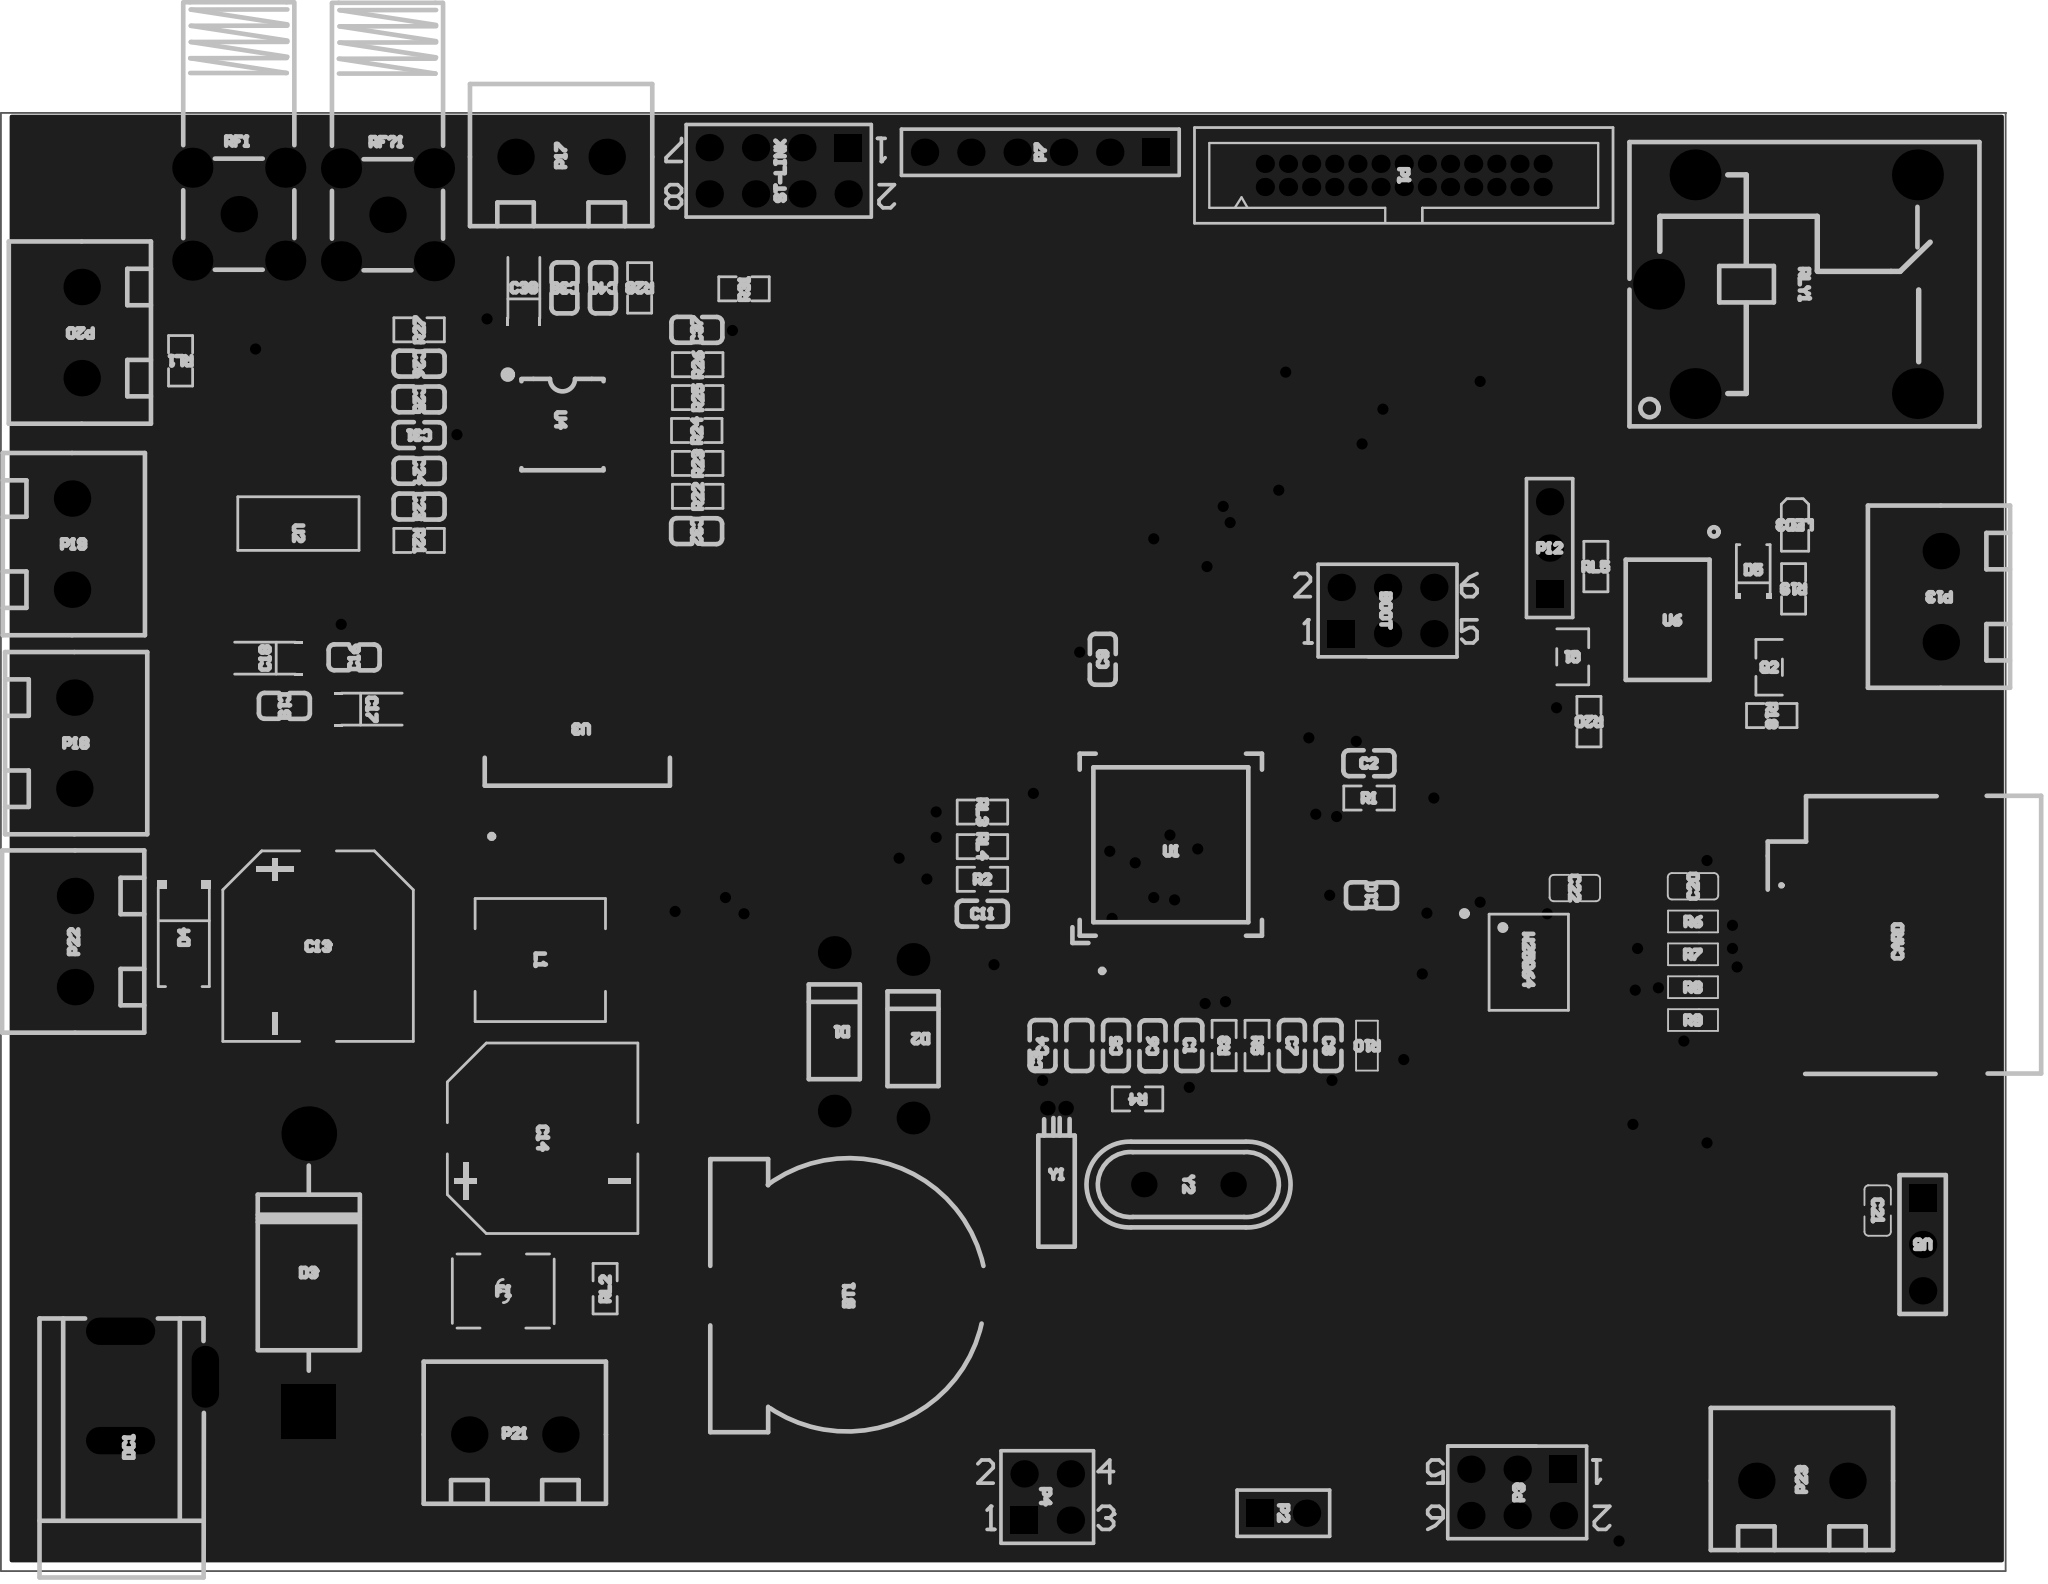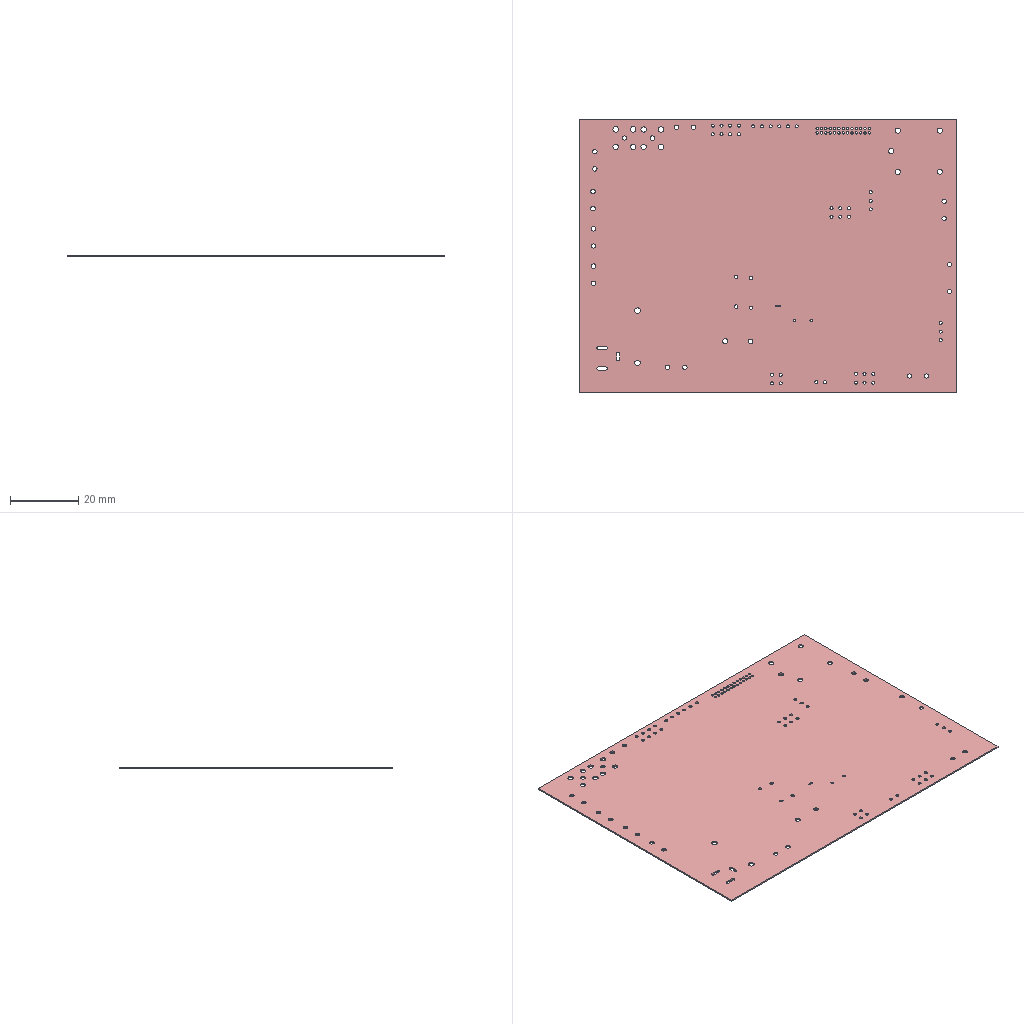Circuit board layout | Altium Designer | box 110 x 80 x 0.4 mm
Layer stack:
# Altium Designer layer stack of  (unit mm; dielectric type: 0 none, 1 core, 2 prepreg, 3 surface material)
index,name,kind,layer,copper_thickness_mm,dielectric_type,dielectric_thickness_mm,dielectric_material,dielectric_constant
0,Top Paste Mask Layer,other,,,,,,
1,Top Silkscreen Layer,other,,,,,,
2,Top Solder Mask Layer,dielectric,,,3,0.0102,Solder Resist,3.5
3,Top Layer,copper,Top Layer,0.0356,,,,
4,Dielectric 1,dielectric,,,3,0.32,FR-4,4.8
5,Bottom Layer,copper,Bottom Layer,0.0356,,,,
6,Bottom Solder Mask Layer,dielectric,,,3,0.0102,Solder Resist,3.5
7,Bottom Silkscreen Layer,other,,,,,,
8,Bottom Paste Mask Layer,other,,,,,,
# drill layer pairs: low layer,high layer
drill_pair,Top Layer,Bottom Layer
Part placement:
Designator,Comment,Layer,Footprint,Center-X(mm),Center-Y(mm),Rotation
Y2,8MHz,TopLayer,OSC-TH_L11.1-W4.7-P4.88,149.352,107.315,0
Y1,32.768kHz,TopLayer,OSC-TH_BD2.0-P0.70-D0.3,142.113,111.506,90
W25Q64,W25Q64JVSSIQ,TopLayer,SOIC-8_L5.3-W5.3-P1.27-LS8.0-BL,168.021,119.514,270
U6,BPC-817SC,TopLayer,OPTO-SMD-4_L4.6-W6.5-P2.54-LS10.3-BR,175.641,138.303,90
U5,DS18B20,TopLayer,H2.54-1X3(RM),189.631,104.025,270
U4,AD8302ARUZ-RL7,TopLayer,TSSOP-14_L5.0-W4.4-P0.65-LS6.4-BL,115.01,149.008,270
U3,LM2596SX-5.0/NOPB,TopLayer,TO-263-5_L10.2-W8.9-P1.70-TL,115.824,131.064,90
U2,LM1117MPX-3.3/NOPB,TopLayer,SOT-223-3_L6.5-W3.4-P2.30-LS7.0-BR,100.522,143.483,270
U1,STM32F103RCT6,TopLayer,TQFP-64_L10.0-W10.0-P0.50-LS12.0-BL,148.385,125.959,0
ST-LINK,Header 4X2,TopLayer,HDR2X4,126.873,162.941,180
RLY1,SRD-05VDC-SL-C,TopLayer,RELAY-TH_SRD-XXVDC-XL-C,182.245,156.718,0
RL5,330,TopLayer,R0603_-_duplicate,171.704,141.224,90
RL4,330,TopLayer,R0603_-_duplicate,138.049,125.857,0
RL3,330,TopLayer,R0603_-_duplicate,138.049,127.755,0
RL2,330,TopLayer,R0603_-_duplicate,117.348,101.6,270
RL1,330,TopLayer,R0603_-_duplicate,94.057,152.514,270
RF1,BWSMA-KWE-Z001,TopLayer,SMA-TH_BWSMA-KWE-Z001,97.251,160.559,90
RF?1,BWSMA-KWE-Z001,TopLayer,SMA-TH_BWSMA-KWE-Z001,105.41,160.528,90
R31,0,TopLayer,R0603,124.968,156.464,180
R28,1K,TopLayer,R0603,119.24,156.515,270
R27,52.3R,TopLayer,R0603,107.143,154.215,180
R26,0,TopLayer,R0603,122.428,152.303,180
R25,100,TopLayer,R0603,122.428,150.497,180
R24,1K,TopLayer,R0603,122.376,148.69,180
R23,100,TopLayer,R0603,122.428,146.884,180
R22,0,TopLayer,R0603,122.428,145.078,180
R21,52.3R,TopLayer,R0603,107.143,142.658,0
R20,10k,TopLayer,R0603_-_duplicate,171.323,132.715,270
R19,10k,TopLayer,R0603_-_duplicate,182.549,140,270
R18,10k,TopLayer,R0603_-_duplicate,181.353,133.049,0
R10,Res,TopLayer,RES[0603],159.131,114.935,270
R9,Res,TopLayer,RES[0603],177.034,116.328,0
R8,Res,TopLayer,RES[0603],177.034,118.132,0
R7,Res,TopLayer,RES[0603],177.034,119.935,0
R6,Res,TopLayer,RES[0603],177.034,121.738,0
R5,10R,TopLayer,R0603,153.114,114.943,270
R4,1M,TopLayer,R0603,146.558,112.014,180
R3,10k,TopLayer,R0603,151.308,114.943,90
R2,10k,TopLayer,R0603,138.049,124.065,0
R1,10k,TopLayer,R0603_-_duplicate,159.258,128.524,0
Q2,MMBT3906,TopLayer,SOT-23-3_L2.9-W1.3-P1.90-LS2.4-BR,181.209,135.698,0
Q1,DTC143ECA,TopLayer,SOT-23-3_L2.9-W1.6-P1.90-LS2.8-BR,170.434,136.271,180
P23,WJ126V-5.0-2P,TopLayer,CONN-TH_WJ126V-5.0-2P,183.007,91.059,90
P22,WJ126V-5.0-2P,TopLayer,CONN-TH_WJ126V-5.0-2P,88.265,120.65,180
P21,WJ126V-5.0-2P,TopLayer,CONN-TH_WJ126V-5.0-2P,112.395,93.599,90
P20,WJ126V-5.0-2P,TopLayer,CONN-TH_WJ126V-5.0-2P,88.633,154.064,180
P19,WJ126V-5.0-2P,TopLayer,CONN-TH_WJ126V-5.0-2P,88.102,142.456,0
P18,WJ126V-5.0-2P,TopLayer,CONN-TH_WJ126V-5.0-2P,88.229,131.534,0
P17,WJ126V-5.0-2P,TopLayer,CONN-TH_WJ126V-5.0-2P,114.935,163.703,90
P13,WJ126V-5.0-2P,TopLayer,CONN-TH_WJ126V-5.0-2P,190.627,139.573,180
P12,Header 3,TopLayer,HDR1X3,169.164,142.24,90
P7,Header 6,TopLayer,HDR1X6,141.224,163.957,180
P4,Header 2X2,TopLayer,HDR2X2,141.605,90.17,0
P3,Header 3X2,TopLayer,HDR2X3,167.386,90.424,180
P2,Header 2,TopLayer,HDR1X2,154.559,89.281,0
LED3,NCD0603R1_C84263,TopLayer,LED0603-RD_RED,182.623,143.457,270
L1,FXL0650-330-M,TopLayer,IND-SMD_L7.0-W6.6_FXL0650,113.792,119.634,180
F1,BSMD1812-150-33V,TopLayer,F1812,111.76,101.473,180
DC1,DC-005-20A_C136744,TopLayer,DC-IN-TH_DC-005-20A,93.091,96.265,90
D5,1N4007W,TopLayer,SOD-123FL_L2.7-W1.8-LS3.8-RD,180.337,141.05,90
D4,1N4007_C727081,TopLayer,SMA_L4.3-W2.5-LS5.0-RD,94.234,120.904,270
D3,1N5822,TopLayer,DO-201AD_BD5.3-L8.4-P12.50-D1.4-FD,101.092,102.489,90
D2,1N4733A_C5157516,TopLayer,DO-41_BD2.4-L4.7-P8.70-D0.9-RD,134.239,115.316,270
D1,1N4733A_C5157516,TopLayer,DO-41_BD2.4-L4.7-P8.70-D0.9-RD,129.921,115.697,270
CARD,TF PUSH,TopLayer,TF-SMD_TF-PUSH,186.432,120.646,90
C40,0.1uF,TopLayer,C0603,117.228,156.507,270
C39,0.1uF,TopLayer,C0603,115.115,156.507,270
C38,10uF,TopLayer,CAP-SMD_L3.2-W1.6-RD-C7171,112.89,156.515,90
C37,0.1uF,TopLayer,C0603,122.376,154.215,180
C32,0.1uF,TopLayer,C0603,122.376,143.166,0
C31,100pF,TopLayer,C0603,107.136,148.439,180
C26,102,TopLayer,C0603,107.151,152.355,0
C25,102,TopLayer,C0603,107.151,150.394,0
C24,102,TopLayer,C0603,107.151,146.473,0
C23,102,TopLayer,C0603,107.151,144.513,0
C22,Cap,TopLayer,CAP[0603],170.561,123.571,0
C21,Cap,TopLayer,CAP[0603],187.15,105.876,270
C20,Cap,TopLayer,CAP[0603],177.019,123.694,180
C19,104,TopLayer,C0603,99.76,133.577,0
C18,TAJA106K016RNJ,TopLayer,CAP-SMD_L3.2-W1.6-RD-C7171,98.698,136.199,180
C17,TAJA106K016RNJ,TopLayer,CAP-SMD_L3.2-W1.6-RD-C7171,104.54,133.402,0
C16,104,TopLayer,C0603,103.57,136.244,180
C14,EEEFK1V331P,TopLayer,CAP-SMD_BD10.0-L10.3-W10.3-FD,113.919,109.855,0
C13,GVM1V681M1010,TopLayer,CAP-SMD_BD10.0-L10.3-W10.3-LS10.9-FD,101.6,120.396,270
C11,104,TopLayer,C0603,138.049,122.174,0
C10,104,TopLayer,C0603,159.385,123.19,180
C9,104,TopLayer,C0603,144.653,136.144,90
C8,104,TopLayer,C0603,157.034,114.935,270
C7,10uF,TopLayer,C0603,155.021,114.935,270
C6,22pF,TopLayer,C0603,147.383,114.935,90
C5,22pF,TopLayer,C0603,145.376,114.951,90
C4,12pF,TopLayer,C0603,141.351,114.951,90
C3,12pF,TopLayer,C0603,143.363,114.951,90
C2,104,TopLayer,C0603,159.258,130.429,0
C1,104,TopLayer,C0603,149.396,114.935,270
BT1,BS-12-B3AA003,TopLayer,BAT-SMD_BS-12-B3AA011,130.556,101.219,180
BOOT,Header 3X2,TopLayer,HDR2X3,160.274,138.811,0
P1,X1270WV-2x13A-6TV01,TopLayer,IDC-TH_X1270WV-2X13A-6TV01,161.163,162.687,0
Pad and via stacks:
# Altium Designer via and pad stacks of  (unit mm). Each distinct definition once, with the count of objects using it.
# via: kind,start_layer,end_layer,hole_mm,diameter_mm,mode(0 simple;1 top-mid-bottom;2 full stack),diameter_per_layer,count,example_net
# pad: kind,layer,hole_mm,hole_type(0 round;1 square;2 slot),plating,top_size,top_shape(1 round;2 rect;3 octagon;9 rounded rect),mid_size,bottom_size,mode,footprint,size_per_layer,count,example
pad,Multi-Layer,0.7,0,plated,1.4x1.4,1,1.4x1.4,1.4x1.4,0,OSC-TH_L11.1-W4.7-P4.88,,2,Y2.2
pad,Multi-Layer,0.5,0,plated,0.8x0.8,1,0.8x0.8,0.8x0.8,0,OSC-TH_BD2.0-P0.70-D0.3,,2,Y1.1
pad,Multi-Layer,0.9,0,plated,1.5x1.5,1,1.5x1.5,1.5x1.5,0,H2.54-1X3(RM),,2,U5.3
pad,Multi-Layer,0.9,0,plated,1.5x1.5,2,1.5x1.5,1.5x1.5,0,H2.54-1X3(RM),,1,U5.1
pad,Multi-Layer,0.9,0,plated,1.5x1.5,1,1.5x1.5,1.5x1.5,0,HDR2X4,,7,ST-LINK.8
pad,Multi-Layer,0.9,0,plated,1.5x1.5,2,1.5x1.5,1.5x1.5,0,HDR2X4,,1,ST-LINK.1
pad,Multi-Layer,1.524,0,plated,2.794x2.794,1,2.794x2.794,2.794x2.794,0,RELAY-TH_SRD-XXVDC-XL-C,,5,RLY1.3
pad,Multi-Layer,1.6,0,plated,2.2x2.2,1,2.2x2.2,2.2x2.2,0,SMA-TH_BWSMA-KWE-Z001,,8,RF1.1
pad,Multi-Layer,1.3,0,plated,2x2,1,2x2,2x2,0,SMA-TH_BWSMA-KWE-Z001,,2,RF1.5
pad,Multi-Layer,1.3,0,plated,2x2,1,2x2,2x2,0,CONN-TH_WJ126V-5.0-2P,,16,P23.2
pad,Multi-Layer,0.9,0,plated,1.5x1.5,2,1.5x1.5,1.5x1.5,0,HDR1X3,,1,P12.1
pad,Multi-Layer,0.9,0,plated,1.5x1.5,1,1.5x1.5,1.5x1.5,0,HDR1X3,,2,P12.2
pad,Multi-Layer,0.9,0,plated,1.5x1.5,2,1.5x1.5,1.5x1.5,0,HDR1X6,,1,P7.1
pad,Multi-Layer,0.9,0,plated,1.5x1.5,1,1.5x1.5,1.5x1.5,0,HDR1X6,,5,P7.2
pad,Multi-Layer,0.9,0,plated,1.5x1.5,1,1.5x1.5,1.5x1.5,0,HDR2X2,,3,P4.4
pad,Multi-Layer,0.9,0,plated,1.5x1.5,2,1.5x1.5,1.5x1.5,0,HDR2X2,,1,P4.1
pad,Multi-Layer,0.9,0,plated,1.5x1.5,2,1.5x1.5,1.5x1.5,0,HDR2X3,,2,P3.1
pad,Multi-Layer,0.9,0,plated,1.5x1.5,1,1.5x1.5,1.5x1.5,0,HDR2X3,,10,P3.2
pad,Multi-Layer,0.9,0,plated,1.5x1.5,2,1.5x1.5,1.5x1.5,0,HDR1X2,,1,P2.1
pad,Multi-Layer,0.9,0,plated,1.5x1.5,1,1.5x1.5,1.5x1.5,0,HDR1X2,,1,P2.2
pad,Multi-Layer,0.9,2,plated,1.5x3.4,1,1.5x3.4,1.5x3.4,0,DC-IN-TH_DC-005-20A,,1,DC1.3
pad,Multi-Layer,0.9,2,plated,1.5x3.8,1,1.5x3.8,1.5x3.8,0,DC-IN-TH_DC-005-20A,,2,DC1.2
pad,Multi-Layer,1.7,0,plated,3x3,1,3x3,3x3,0,DO-201AD_BD5.3-L8.4-P12.50-D1.4-FD,,1,D3.2
pad,Multi-Layer,1.7,0,plated,3x3,2,3x3,3x3,0,DO-201AD_BD5.3-L8.4-P12.50-D1.4-FD,,1,D3.1
pad,Multi-Layer,1,0,plated,1.8x1.8,1,1.8x1.8,1.8x1.8,0,DO-41_BD2.4-L4.7-P8.70-D0.9-RD,,4,D2.1
pad,Multi-Layer,0.7,0,plated,1x1,1,1x1,1x1,0,IDC-TH_X1270WV-2X13A-6TV01,,26,P1.1
pad,Top Layer,0,0,plated,0.63x2.25,1,0.63x2.25,0.63x2.25,0,SOIC-8_L5.3-W5.3-P1.27-LS8.0-BL,,8,W25Q64.1
pad,Top Layer,0,0,plated,1.5x3,2,1.5x3,1.5x3,0,OPTO-SMD-4_L4.6-W6.5-P2.54-LS10.3-BR,,4,U6.1
pad,Top Layer,0,0,plated,0.4x1.7,2,0.4x1.7,0.4x1.7,0,TSSOP-14_L5.0-W4.4-P0.65-LS6.4-BL,,14,U4.1
pad,Top Layer,0,0,plated,8.128x10.922,1,8.128x10.922,8.128x10.922,0,TO-263-5_L10.2-W8.9-P1.70-TL,,1,U3.6
pad,Top Layer,0,0,plated,3.2x1.15,2,3.2x1.15,3.2x1.15,0,TO-263-5_L10.2-W8.9-P1.70-TL,,5,U3.1
pad,Top Layer,0,0,plated,2.5x1.1,2,2.5x1.1,2.5x1.1,0,SOT-223-3_L6.5-W3.4-P2.30-LS7.0-BR,,3,U2.1
pad,Top Layer,0,0,plated,2.34x3.6,2,2.34x3.6,2.34x3.6,0,SOT-223-3_L6.5-W3.4-P2.30-LS7.0-BR,,1,U2.4
pad,Top Layer,0,0,plated,1.8x0.28,1,1.8x0.28,1.8x0.28,0,TQFP-64_L10.0-W10.0-P0.50-LS12.0-BL,,32,U1.64
pad,Top Layer,0,0,plated,0.28x1.8,1,0.28x1.8,0.28x1.8,0,TQFP-64_L10.0-W10.0-P0.50-LS12.0-BL,,32,U1.48
pad,Top Layer,0,0,plated,0.8065x0.864,2,0.8065x0.864,0.8065x0.864,0,R0603 - duplicate,,18,RL5.2
pad,Top Layer,0,0,plated,0.8065x0.864,2,0.8065x0.864,0.8065x0.864,0,R0603,,26,R31.2
pad,Top Layer,0,0,plated,0.8x0.965,2,0.8x0.965,0.8x0.965,0,RES[0603],,10,R10.1
pad,Top Layer,0,0,plated,1.25x0.7,2,1.25x0.7,1.25x0.7,0,SOT-23-3_L2.9-W1.3-P1.90-LS2.4-BR,,3,Q2.3
pad,Top Layer,0,0,plated,1.07x0.6,2,1.07x0.6,1.07x0.6,0,SOT-23-3_L2.9-W1.6-P1.90-LS2.8-BR,,3,Q1.1
pad,Top Layer,0,0,plated,0.8x0.8,2,0.8x0.8,0.8x0.8,0,LED0603-RD_RED,,2,LED3.1
pad,Top Layer,0,0,plated,2.524x3.5,2,2.524x3.5,2.524x3.5,0,IND-SMD_L7.0-W6.6_FXL0650,,2,L1.2
pad,Top Layer,0,0,plated,1.407x3.499,2,1.407x3.499,1.407x3.499,0,F1812,,2,F1.2
pad,Top Layer,0,0,plated,1.4x1.2,2,1.4x1.2,1.4x1.2,0,SOD-123FL_L2.7-W1.8-LS3.8-RD,,2,D5.2
pad,Top Layer,0,0,plated,2x1.593,2,2x1.593,2x1.593,0,SMA_L4.3-W2.5-LS5.0-RD,,2,D4.2
pad,Top Layer,0,0,plated,1.6x1.5,2,1.6x1.5,1.6x1.5,0,TF-SMD_TF-PUSH,,1,CARD.13
pad,Top Layer,0,0,plated,1.2x2.2,2,1.2x2.2,1.2x2.2,0,TF-SMD_TF-PUSH,,2,CARD.12
pad,Top Layer,0,0,plated,1.2x1.5,2,1.2x1.5,1.2x1.5,0,TF-SMD_TF-PUSH,,1,CARD.10
pad,Top Layer,0,0,plated,0.7x1.6,2,0.7x1.6,0.7x1.6,0,TF-SMD_TF-PUSH,,9,CARD.CD
pad,Top Layer,0,0,plated,0.8x0.9,2,0.8x0.9,0.8x0.9,0,C0603,,44,C40.1
pad,Top Layer,0,0,plated,1.758x1.296,2,1.758x1.296,1.758x1.296,0,CAP-SMD_L3.2-W1.6-RD-C7171,,6,C38.1
pad,Top Layer,0,0,plated,0.8x0.965,2,0.8x0.965,0.8x0.965,0,CAP[0603],,6,C22.2
pad,Top Layer,0,0,plated,4.5x1.65,2,4.5x1.65,4.5x1.65,0,CAP-SMD_BD10.0-L10.3-W10.3-FD,,2,C14.1
pad,Top Layer,0,0,plated,4.5x1.65,2,4.5x1.65,4.5x1.65,0,CAP-SMD_BD10.0-L10.3-W10.3-LS10.9-FD,,2,C13.1
pad,Top Layer,0,0,plated,3.75x2.8,2,3.75x2.8,3.75x2.8,0,BAT-SMD_BS-12-B3AA011,,1,BT1.1
pad,Top Layer,0,0,plated,4.4x2.8,2,4.4x2.8,4.4x2.8,0,BAT-SMD_BS-12-B3AA011,,1,BT1.2
via,Top Layer,Bottom Layer,0.3048,0.61,0,,61,PA5
Copper pours:
name,layer,net,type(0 solid;1 hatched;2 none)
Top Layer-GND,Top Layer,GND,0
Top Layer-AGND,Top Layer,AGND,0
Bottom Layer-GND,Bottom Layer,GND,0
Bottom Layer-AGND,Bottom Layer,AGND,0
Design rules, without the lines most boards share:
# Altium Designer design rules of  (exported by Altium Designer, unit mm)
# columns: name | kind | enabled | priority | scope1 | scope2 | descriptor | typed fields (field=value)
ComponentClearance_1 | 24 | enabled | 1 | All | All | Component Clearance Constraint ( Horizontal Gap = 10mil, Vertical Gap = 10mil ) (All),(All)  | gap=0.254
Clearance | 0 | enabled | 1 | All | All | Clearance Constraint (Gap=4mil) (All),(All) | gap=0.1016
Clearance_1 | 63 | enabled | 1 | All | All | Board Clearance Constraint (Gap=0mil) (All) |
ComponentClearance | 52 | enabled | 1 | All | All | Hole To Hole Clearance (Gap=10mil) (All),(All) | gap=0.254
Width | 2 | enabled | 1 | All | All | Width Constraint (Min=10mil) (Max=300mil) (Preferred=10mil) (All) |
DiffPairsRouting | 51 | enabled | 1 | All | All | Differential Pairs Uncoupled Length using the Gap Constraints (Min=10mil) (Max=10mil) (Prefered=10mil)  and Width Constraints (Min=15mil) (Max=15mil) (Prefered=15mil) (All) |
RoutingVias | 11 | enabled | 1 | All | All | Routing Via (MinHoleWidth=1mil) (MaxHoleWidth=28mil) (PreferredHoleWidth=12mil) (MinWidth=1mil) (MaxWidth=50mil) (PreferedWidth=24mil) (All) | via_min_hole=0.0254 via_max_hole=0.7112 via_preferred_diameter=0.6096 via_preferred_hole=0.3048
PlaneConnect | 6 | enabled | 1 | All | All | Power Plane Connect Rule(Relief Connect )(Expansion=20mil) (Conductor Width=10mil) (Air Gap=10mil) (Entries=4) (All) | relief_conductor_width=0.254 relief_entries=4 relief_expansion=0.508
PolygonConnect | 20 | enabled | 1 | (InNet('AGND') OR InNet('GND')) | All | Polygon Connect Rule(Relief Connect )(Conductor Width=10mil) (Relief Angle=90 Angle) (Entries=4) (Air Gap Width=10mil) ((InNet('AGND') OR InNet('GND'))),(All) | connect_style(0=relief,1=direct,2=none)=0 relief_conductor_width=0.254 relief_entries=4
PasteMaskExpansion | 14 | enabled | 1 | All | All | Paste Mask Expansion (Expansion =0mil) (All) | expansion=0
SolderMaskExpansion | 13 | enabled | 1 | All | All | Solder Mask Expansion (Expansion =4mil) (All) | expansion=0.1016